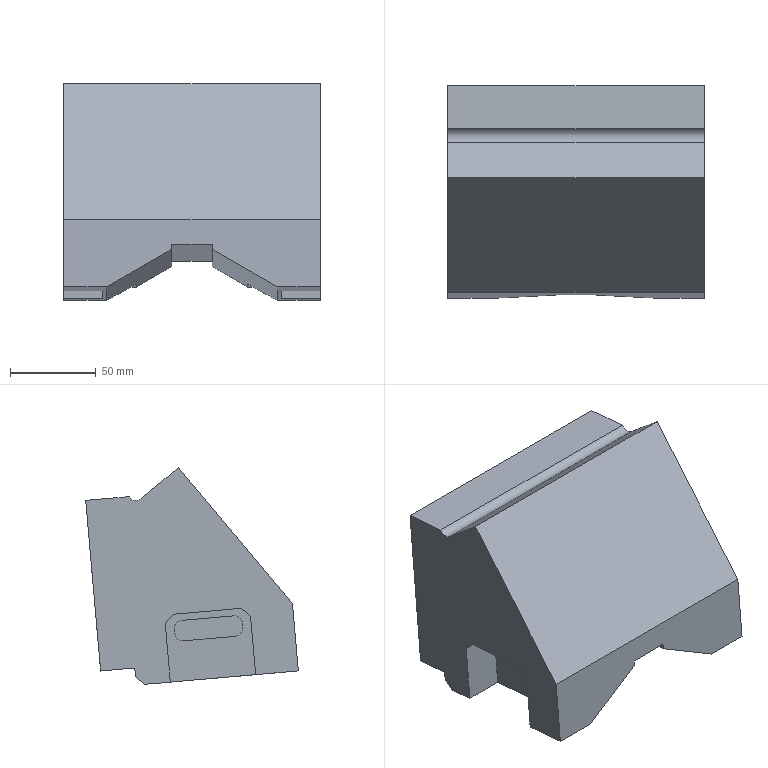Part | NX | features solid 2 | 1 solid | 51 faces | box 150 x 124.15 x 126.523 mm | volume 1390893 mm3 | plane 42 | cylinder 9 | commonest cylinder face diameters 10 x9